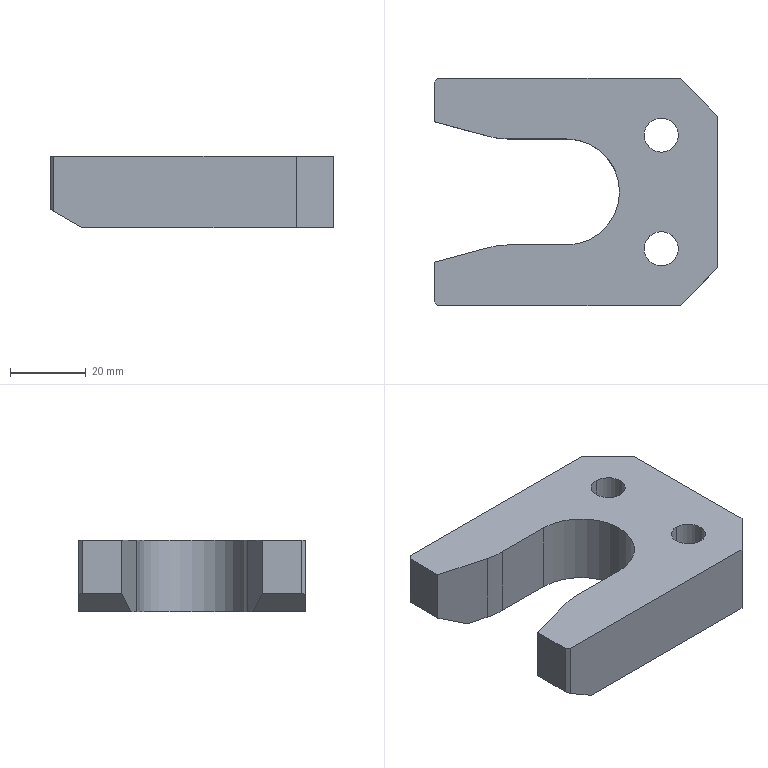Part | 1 solid | 30 faces | box 75 x 60 x 19 mm | volume 52700 mm3 | plane 19 | cylinder 11 | commonest cylinder face diameters 9 x4 14 x4 40 x2 28 x1